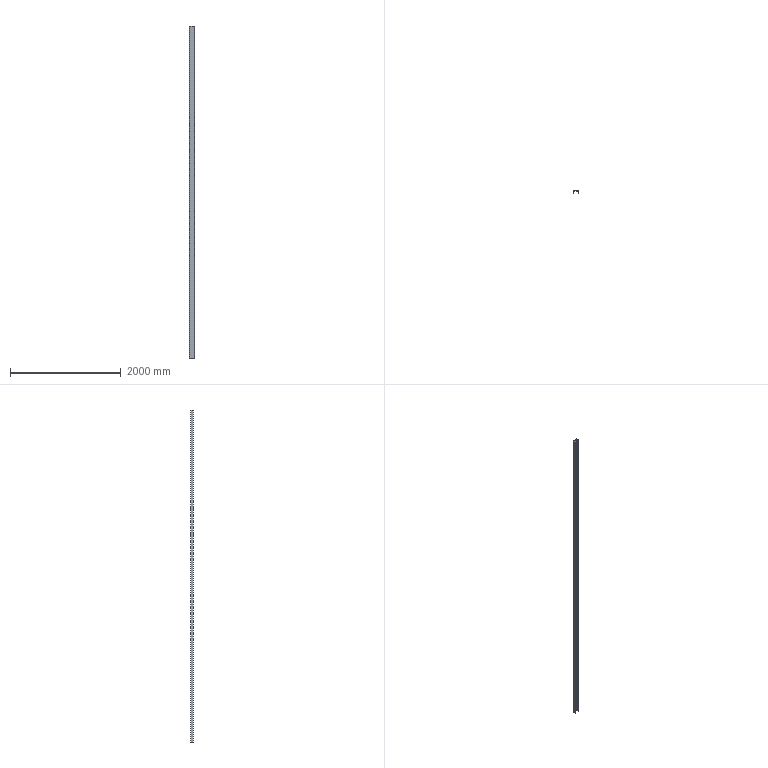Part | SolidWorks | features Extrusion 1 | 1 solid | 14 faces | box 100 x 50 x 6000 mm | volume 7666640 mm3 | plane 10 | cylinder 4 | commonest cylinder face diameters 4 x2 10 x2
STEP:
#1=CARTESIAN_POINT('',(0.,0.,0.));
#2=VERTEX_POINT('',#1);
#3=CARTESIAN_POINT('',(2.549,0.,0.));
#4=VERTEX_POINT('',#3);
#5=CARTESIAN_POINT('',(0.,0.,0.));
#6=DIRECTION('',(1.,0.,0.));
#7=VECTOR('',#6,1000.);
#8=LINE('',#5,#7);
#9=EDGE_CURVE('',#2,#4,#8,.T.);
#10=ORIENTED_EDGE('',*,*,#9,.T.);
#11=CARTESIAN_POINT('',(2.549,0.,6000.));
#12=VERTEX_POINT('',#11);
#13=CARTESIAN_POINT('',(2.549,0.,6000.));
#14=DIRECTION('',(0.,0.,-1.));
#15=VECTOR('',#14,1000.);
#16=LINE('',#13,#15);
#17=EDGE_CURVE('',#12,#4,#16,.T.);
#18=ORIENTED_EDGE('',*,*,#17,.F.);
#19=CARTESIAN_POINT('',(0.,0.,6000.));
#20=VERTEX_POINT('',#19);
#21=CARTESIAN_POINT('',(0.,0.,6000.));
#22=DIRECTION('',(1.,0.,0.));
#23=VECTOR('',#22,1000.);
#24=LINE('',#21,#23);
#25=EDGE_CURVE('',#20,#12,#24,.T.);
#26=ORIENTED_EDGE('',*,*,#25,.F.);
#27=CARTESIAN_POINT('',(0.,0.,6000.));
#28=DIRECTION('',(0.,0.,-1.));
#29=VECTOR('',#28,1000.);
#30=LINE('',#27,#29);
#31=EDGE_CURVE('',#20,#2,#30,.T.);
#32=ORIENTED_EDGE('',*,*,#31,.T.);
#33=EDGE_LOOP('',(#10,#18,#26,#32));
#34=FACE_OUTER_BOUND('',#33,.T.);
#35=CARTESIAN_POINT('',(0.,0.,6000.));
#36=DIRECTION('',(0.,1.,0.));
#37=DIRECTION('',(0.,0.,1.));
#38=AXIS2_PLACEMENT_3D('',#35,#36,#37);
#39=PLANE('',#38);
#40=ADVANCED_FACE('',(#34),#39,.F.);
#41=CARTESIAN_POINT('',(4.536,1.773,0.));
#42=VERTEX_POINT('',#41);
#43=CARTESIAN_POINT('',(2.549,2.,0.));
#44=DIRECTION('',(0.,0.,1.));
#45=DIRECTION('',(-1.,0.,0.));
#46=AXIS2_PLACEMENT_3D('',#43,#44,#45);
#47=CIRCLE('',#46,2.);
#48=EDGE_CURVE('',#4,#42,#47,.T.);
#49=ORIENTED_EDGE('',*,*,#48,.T.);
#50=CARTESIAN_POINT('',(4.536,1.773,6000.));
#51=VERTEX_POINT('',#50);
#52=CARTESIAN_POINT('',(4.536,1.773,6000.));
#53=DIRECTION('',(0.,0.,-1.));
#54=VECTOR('',#53,1000.);
#55=LINE('',#52,#54);
#56=EDGE_CURVE('',#51,#42,#55,.T.);
#57=ORIENTED_EDGE('',*,*,#56,.F.);
#58=CARTESIAN_POINT('',(2.549,2.,6000.));
#59=DIRECTION('',(0.,0.,1.));
#60=DIRECTION('',(-1.,0.,0.));
#61=AXIS2_PLACEMENT_3D('',#58,#59,#60);
#62=CIRCLE('',#61,2.);
#63=EDGE_CURVE('',#12,#51,#62,.T.);
#64=ORIENTED_EDGE('',*,*,#63,.F.);
#65=ORIENTED_EDGE('',*,*,#17,.T.);
#66=EDGE_LOOP('',(#49,#57,#64,#65));
#67=FACE_OUTER_BOUND('',#66,.T.);
#68=CARTESIAN_POINT('',(2.549,2.,6000.));
#69=DIRECTION('',(0.,0.,-1.));
#70=DIRECTION('',(-1.,0.,0.));
#71=AXIS2_PLACEMENT_3D('',#68,#69,#70);
#72=CYLINDRICAL_SURFACE('',#71,2.);
#73=ADVANCED_FACE('',(#67),#72,.T.);
#74=CARTESIAN_POINT('',(8.753,38.724,0.));
#75=VERTEX_POINT('',#74);
#76=CARTESIAN_POINT('',(4.536,1.773,0.));
#77=DIRECTION('',(0.1134,0.9936,0.));
#78=VECTOR('',#77,1000.);
#79=LINE('',#76,#78);
#80=EDGE_CURVE('',#42,#75,#79,.T.);
#81=ORIENTED_EDGE('',*,*,#80,.T.);
#82=CARTESIAN_POINT('',(8.753,38.724,6000.));
#83=VERTEX_POINT('',#82);
#84=CARTESIAN_POINT('',(8.753,38.724,6000.));
#85=DIRECTION('',(0.,0.,-1.));
#86=VECTOR('',#85,1000.);
#87=LINE('',#84,#86);
#88=EDGE_CURVE('',#83,#75,#87,.T.);
#89=ORIENTED_EDGE('',*,*,#88,.F.);
#90=CARTESIAN_POINT('',(4.536,1.773,6000.));
#91=DIRECTION('',(0.1134,0.9936,0.));
#92=VECTOR('',#91,1000.);
#93=LINE('',#90,#92);
#94=EDGE_CURVE('',#51,#83,#93,.T.);
#95=ORIENTED_EDGE('',*,*,#94,.F.);
#96=ORIENTED_EDGE('',*,*,#56,.T.);
#97=EDGE_LOOP('',(#81,#89,#95,#96));
#98=FACE_OUTER_BOUND('',#97,.T.);
#99=CARTESIAN_POINT('',(4.536,1.773,6000.));
#100=DIRECTION('',(-0.9936,0.1134,0.));
#101=DIRECTION('',(-0.1134,-0.9936,0.));
#102=AXIS2_PLACEMENT_3D('',#99,#100,#101);
#103=PLANE('',#102);
#104=ADVANCED_FACE('',(#98),#103,.F.);
#105=CARTESIAN_POINT('',(13.72,43.157,0.));
#106=VERTEX_POINT('',#105);
#107=CARTESIAN_POINT('',(13.72,38.157,0.));
#108=DIRECTION('',(0.,0.,-1.));
#109=DIRECTION('',(-1.,0.,0.));
#110=AXIS2_PLACEMENT_3D('',#107,#108,#109);
#111=CIRCLE('',#110,5.);
#112=EDGE_CURVE('',#75,#106,#111,.T.);
#113=ORIENTED_EDGE('',*,*,#112,.T.);
#114=CARTESIAN_POINT('',(13.72,43.157,6000.));
#115=VERTEX_POINT('',#114);
#116=CARTESIAN_POINT('',(13.72,43.157,6000.));
#117=DIRECTION('',(0.,0.,-1.));
#118=VECTOR('',#117,1000.);
#119=LINE('',#116,#118);
#120=EDGE_CURVE('',#115,#106,#119,.T.);
#121=ORIENTED_EDGE('',*,*,#120,.F.);
#122=CARTESIAN_POINT('',(13.72,38.157,6000.));
#123=DIRECTION('',(0.,0.,-1.));
#124=DIRECTION('',(-1.,0.,0.));
#125=AXIS2_PLACEMENT_3D('',#122,#123,#124);
#126=CIRCLE('',#125,5.);
#127=EDGE_CURVE('',#83,#115,#126,.T.);
#128=ORIENTED_EDGE('',*,*,#127,.F.);
#129=ORIENTED_EDGE('',*,*,#88,.T.);
#130=EDGE_LOOP('',(#113,#121,#128,#129));
#131=FACE_OUTER_BOUND('',#130,.T.);
#132=CARTESIAN_POINT('',(13.72,38.157,6000.));
#133=DIRECTION('',(0.,0.,-1.));
#134=DIRECTION('',(-1.,0.,0.));
#135=AXIS2_PLACEMENT_3D('',#132,#133,#134);
#136=CYLINDRICAL_SURFACE('',#135,5.);
#137=ADVANCED_FACE('',(#131),#136,.F.);
#138=CARTESIAN_POINT('',(86.28,43.157,0.));
#139=VERTEX_POINT('',#138);
#140=CARTESIAN_POINT('',(13.72,43.157,0.));
#141=DIRECTION('',(1.,0.,0.));
#142=VECTOR('',#141,1000.);
#143=LINE('',#140,#142);
#144=EDGE_CURVE('',#106,#139,#143,.T.);
#145=ORIENTED_EDGE('',*,*,#144,.T.);
#146=CARTESIAN_POINT('',(86.28,43.157,6000.));
#147=VERTEX_POINT('',#146);
#148=CARTESIAN_POINT('',(86.28,43.157,6000.));
#149=DIRECTION('',(0.,0.,-1.));
#150=VECTOR('',#149,1000.);
#151=LINE('',#148,#150);
#152=EDGE_CURVE('',#147,#139,#151,.T.);
#153=ORIENTED_EDGE('',*,*,#152,.F.);
#154=CARTESIAN_POINT('',(13.72,43.157,6000.));
#155=DIRECTION('',(1.,0.,0.));
#156=VECTOR('',#155,1000.);
#157=LINE('',#154,#156);
#158=EDGE_CURVE('',#115,#147,#157,.T.);
#159=ORIENTED_EDGE('',*,*,#158,.F.);
#160=ORIENTED_EDGE('',*,*,#120,.T.);
#161=EDGE_LOOP('',(#145,#153,#159,#160));
#162=FACE_OUTER_BOUND('',#161,.T.);
#163=CARTESIAN_POINT('',(13.72,43.157,6000.));
#164=DIRECTION('',(0.,1.,0.));
#165=DIRECTION('',(-1.,0.,0.));
#166=AXIS2_PLACEMENT_3D('',#163,#164,#165);
#167=PLANE('',#166);
#168=ADVANCED_FACE('',(#162),#167,.F.);
#169=CARTESIAN_POINT('',(91.247,38.724,0.));
#170=VERTEX_POINT('',#169);
#171=CARTESIAN_POINT('',(86.28,38.157,0.));
#172=DIRECTION('',(0.,0.,-1.));
#173=DIRECTION('',(1.,0.,0.));
#174=AXIS2_PLACEMENT_3D('',#171,#172,#173);
#175=CIRCLE('',#174,5.);
#176=EDGE_CURVE('',#139,#170,#175,.T.);
#177=ORIENTED_EDGE('',*,*,#176,.T.);
#178=CARTESIAN_POINT('',(91.247,38.724,6000.));
#179=VERTEX_POINT('',#178);
#180=CARTESIAN_POINT('',(91.247,38.724,6000.));
#181=DIRECTION('',(0.,0.,-1.));
#182=VECTOR('',#181,1000.);
#183=LINE('',#180,#182);
#184=EDGE_CURVE('',#179,#170,#183,.T.);
#185=ORIENTED_EDGE('',*,*,#184,.F.);
#186=CARTESIAN_POINT('',(86.28,38.157,6000.));
#187=DIRECTION('',(0.,0.,-1.));
#188=DIRECTION('',(1.,0.,0.));
#189=AXIS2_PLACEMENT_3D('',#186,#187,#188);
#190=CIRCLE('',#189,5.);
#191=EDGE_CURVE('',#147,#179,#190,.T.);
#192=ORIENTED_EDGE('',*,*,#191,.F.);
#193=ORIENTED_EDGE('',*,*,#152,.T.);
#194=EDGE_LOOP('',(#177,#185,#192,#193));
#195=FACE_OUTER_BOUND('',#194,.T.);
#196=CARTESIAN_POINT('',(86.28,38.157,6000.));
#197=DIRECTION('',(0.,0.,-1.));
#198=DIRECTION('',(-1.,0.,0.));
#199=AXIS2_PLACEMENT_3D('',#196,#197,#198);
#200=CYLINDRICAL_SURFACE('',#199,5.);
#201=ADVANCED_FACE('',(#195),#200,.F.);
#202=CARTESIAN_POINT('',(95.464,1.773,0.));
#203=VERTEX_POINT('',#202);
#204=CARTESIAN_POINT('',(95.464,1.773,0.));
#205=DIRECTION('',(0.1134,-0.9936,0.));
#206=VECTOR('',#205,1000.);
#207=LINE('',#204,#206);
#208=EDGE_CURVE('',#170,#203,#207,.T.);
#209=ORIENTED_EDGE('',*,*,#208,.T.);
#210=CARTESIAN_POINT('',(95.464,1.773,6000.));
#211=VERTEX_POINT('',#210);
#212=CARTESIAN_POINT('',(95.464,1.773,6000.));
#213=DIRECTION('',(0.,0.,-1.));
#214=VECTOR('',#213,1000.);
#215=LINE('',#212,#214);
#216=EDGE_CURVE('',#211,#203,#215,.T.);
#217=ORIENTED_EDGE('',*,*,#216,.F.);
#218=CARTESIAN_POINT('',(95.464,1.773,6000.));
#219=DIRECTION('',(0.1134,-0.9936,0.));
#220=VECTOR('',#219,1000.);
#221=LINE('',#218,#220);
#222=EDGE_CURVE('',#179,#211,#221,.T.);
#223=ORIENTED_EDGE('',*,*,#222,.F.);
#224=ORIENTED_EDGE('',*,*,#184,.T.);
#225=EDGE_LOOP('',(#209,#217,#223,#224));
#226=FACE_OUTER_BOUND('',#225,.T.);
#227=CARTESIAN_POINT('',(95.464,1.773,6000.));
#228=DIRECTION('',(0.9936,0.1134,0.));
#229=DIRECTION('',(-0.1134,0.9936,0.));
#230=AXIS2_PLACEMENT_3D('',#227,#228,#229);
#231=PLANE('',#230);
#232=ADVANCED_FACE('',(#226),#231,.F.);
#233=CARTESIAN_POINT('',(97.451,0.,0.));
#234=VERTEX_POINT('',#233);
#235=CARTESIAN_POINT('',(97.451,2.,0.));
#236=DIRECTION('',(0.,0.,1.));
#237=DIRECTION('',(1.,0.,0.));
#238=AXIS2_PLACEMENT_3D('',#235,#236,#237);
#239=CIRCLE('',#238,2.);
#240=EDGE_CURVE('',#203,#234,#239,.T.);
#241=ORIENTED_EDGE('',*,*,#240,.T.);
#242=CARTESIAN_POINT('',(97.451,0.,6000.));
#243=VERTEX_POINT('',#242);
#244=CARTESIAN_POINT('',(97.451,0.,6000.));
#245=DIRECTION('',(0.,0.,-1.));
#246=VECTOR('',#245,1000.);
#247=LINE('',#244,#246);
#248=EDGE_CURVE('',#243,#234,#247,.T.);
#249=ORIENTED_EDGE('',*,*,#248,.F.);
#250=CARTESIAN_POINT('',(97.451,2.,6000.));
#251=DIRECTION('',(0.,0.,1.));
#252=DIRECTION('',(1.,0.,0.));
#253=AXIS2_PLACEMENT_3D('',#250,#251,#252);
#254=CIRCLE('',#253,2.);
#255=EDGE_CURVE('',#211,#243,#254,.T.);
#256=ORIENTED_EDGE('',*,*,#255,.F.);
#257=ORIENTED_EDGE('',*,*,#216,.T.);
#258=EDGE_LOOP('',(#241,#249,#256,#257));
#259=FACE_OUTER_BOUND('',#258,.T.);
#260=CARTESIAN_POINT('',(97.451,2.,6000.));
#261=DIRECTION('',(0.,0.,-1.));
#262=DIRECTION('',(-1.,0.,0.));
#263=AXIS2_PLACEMENT_3D('',#260,#261,#262);
#264=CYLINDRICAL_SURFACE('',#263,2.);
#265=ADVANCED_FACE('',(#259),#264,.T.);
#266=CARTESIAN_POINT('',(100.,0.,0.));
#267=VERTEX_POINT('',#266);
#268=CARTESIAN_POINT('',(100.,0.,0.));
#269=DIRECTION('',(1.,0.,0.));
#270=VECTOR('',#269,1000.);
#271=LINE('',#268,#270);
#272=EDGE_CURVE('',#234,#267,#271,.T.);
#273=ORIENTED_EDGE('',*,*,#272,.T.);
#274=CARTESIAN_POINT('',(100.,0.,6000.));
#275=VERTEX_POINT('',#274);
#276=CARTESIAN_POINT('',(100.,0.,6000.));
#277=DIRECTION('',(0.,0.,-1.));
#278=VECTOR('',#277,1000.);
#279=LINE('',#276,#278);
#280=EDGE_CURVE('',#275,#267,#279,.T.);
#281=ORIENTED_EDGE('',*,*,#280,.F.);
#282=CARTESIAN_POINT('',(100.,0.,6000.));
#283=DIRECTION('',(1.,0.,0.));
#284=VECTOR('',#283,1000.);
#285=LINE('',#282,#284);
#286=EDGE_CURVE('',#243,#275,#285,.T.);
#287=ORIENTED_EDGE('',*,*,#286,.F.);
#288=ORIENTED_EDGE('',*,*,#248,.T.);
#289=EDGE_LOOP('',(#273,#281,#287,#288));
#290=FACE_OUTER_BOUND('',#289,.T.);
#291=CARTESIAN_POINT('',(100.,0.,6000.));
#292=DIRECTION('',(0.,1.,0.));
#293=DIRECTION('',(-1.,0.,0.));
#294=AXIS2_PLACEMENT_3D('',#291,#292,#293);
#295=PLANE('',#294);
#296=ADVANCED_FACE('',(#290),#295,.F.);
#297=CARTESIAN_POINT('',(100.,50.,0.));
#298=VERTEX_POINT('',#297);
#299=CARTESIAN_POINT('',(100.,50.,0.));
#300=DIRECTION('',(0.,1.,0.));
#301=VECTOR('',#300,1000.);
#302=LINE('',#299,#301);
#303=EDGE_CURVE('',#267,#298,#302,.T.);
#304=ORIENTED_EDGE('',*,*,#303,.T.);
#305=CARTESIAN_POINT('',(100.,50.,6000.));
#306=VERTEX_POINT('',#305);
#307=CARTESIAN_POINT('',(100.,50.,6000.));
#308=DIRECTION('',(0.,0.,-1.));
#309=VECTOR('',#308,1000.);
#310=LINE('',#307,#309);
#311=EDGE_CURVE('',#306,#298,#310,.T.);
#312=ORIENTED_EDGE('',*,*,#311,.F.);
#313=CARTESIAN_POINT('',(100.,50.,6000.));
#314=DIRECTION('',(0.,1.,0.));
#315=VECTOR('',#314,1000.);
#316=LINE('',#313,#315);
#317=EDGE_CURVE('',#275,#306,#316,.T.);
#318=ORIENTED_EDGE('',*,*,#317,.F.);
#319=ORIENTED_EDGE('',*,*,#280,.T.);
#320=EDGE_LOOP('',(#304,#312,#318,#319));
#321=FACE_OUTER_BOUND('',#320,.T.);
#322=CARTESIAN_POINT('',(100.,50.,6000.));
#323=DIRECTION('',(-1.,0.,0.));
#324=DIRECTION('',(0.,-1.,0.));
#325=AXIS2_PLACEMENT_3D('',#322,#323,#324);
#326=PLANE('',#325);
#327=ADVANCED_FACE('',(#321),#326,.F.);
#328=CARTESIAN_POINT('',(0.,50.,0.));
#329=VERTEX_POINT('',#328);
#330=CARTESIAN_POINT('',(0.,50.,0.));
#331=DIRECTION('',(-1.,0.,0.));
#332=VECTOR('',#331,1000.);
#333=LINE('',#330,#332);
#334=EDGE_CURVE('',#298,#329,#333,.T.);
#335=ORIENTED_EDGE('',*,*,#334,.T.);
#336=CARTESIAN_POINT('',(0.,50.,6000.));
#337=VERTEX_POINT('',#336);
#338=CARTESIAN_POINT('',(0.,50.,6000.));
#339=DIRECTION('',(0.,0.,-1.));
#340=VECTOR('',#339,1000.);
#341=LINE('',#338,#340);
#342=EDGE_CURVE('',#337,#329,#341,.T.);
#343=ORIENTED_EDGE('',*,*,#342,.F.);
#344=CARTESIAN_POINT('',(0.,50.,6000.));
#345=DIRECTION('',(-1.,0.,0.));
#346=VECTOR('',#345,1000.);
#347=LINE('',#344,#346);
#348=EDGE_CURVE('',#306,#337,#347,.T.);
#349=ORIENTED_EDGE('',*,*,#348,.F.);
#350=ORIENTED_EDGE('',*,*,#311,.T.);
#351=EDGE_LOOP('',(#335,#343,#349,#350));
#352=FACE_OUTER_BOUND('',#351,.T.);
#353=CARTESIAN_POINT('',(0.,50.,6000.));
#354=DIRECTION('',(0.,-1.,0.));
#355=DIRECTION('',(1.,0.,0.));
#356=AXIS2_PLACEMENT_3D('',#353,#354,#355);
#357=PLANE('',#356);
#358=ADVANCED_FACE('',(#352),#357,.F.);
#359=CARTESIAN_POINT('',(0.,0.,0.));
#360=DIRECTION('',(0.,-1.,0.));
#361=VECTOR('',#360,1000.);
#362=LINE('',#359,#361);
#363=EDGE_CURVE('',#329,#2,#362,.T.);
#364=ORIENTED_EDGE('',*,*,#363,.T.);
#365=ORIENTED_EDGE('',*,*,#31,.F.);
#366=CARTESIAN_POINT('',(0.,0.,6000.));
#367=DIRECTION('',(0.,-1.,0.));
#368=VECTOR('',#367,1000.);
#369=LINE('',#366,#368);
#370=EDGE_CURVE('',#337,#20,#369,.T.);
#371=ORIENTED_EDGE('',*,*,#370,.F.);
#372=ORIENTED_EDGE('',*,*,#342,.T.);
#373=EDGE_LOOP('',(#364,#365,#371,#372));
#374=FACE_OUTER_BOUND('',#373,.T.);
#375=CARTESIAN_POINT('',(0.,0.,6000.));
#376=DIRECTION('',(1.,0.,0.));
#377=DIRECTION('',(0.,0.,-1.));
#378=AXIS2_PLACEMENT_3D('',#375,#376,#377);
#379=PLANE('',#378);
#380=ADVANCED_FACE('',(#374),#379,.F.);
#381=ORIENTED_EDGE('',*,*,#25,.T.);
#382=ORIENTED_EDGE('',*,*,#63,.T.);
#383=ORIENTED_EDGE('',*,*,#94,.T.);
#384=ORIENTED_EDGE('',*,*,#127,.T.);
#385=ORIENTED_EDGE('',*,*,#158,.T.);
#386=ORIENTED_EDGE('',*,*,#191,.T.);
#387=ORIENTED_EDGE('',*,*,#222,.T.);
#388=ORIENTED_EDGE('',*,*,#255,.T.);
#389=ORIENTED_EDGE('',*,*,#286,.T.);
#390=ORIENTED_EDGE('',*,*,#317,.T.);
#391=ORIENTED_EDGE('',*,*,#348,.T.);
#392=ORIENTED_EDGE('',*,*,#370,.T.);
#393=EDGE_LOOP('',(#381,#382,#383,#384,#385,#386,#387,#388,#389,#390,#391,#392));
#394=FACE_OUTER_BOUND('',#393,.T.);
#395=CARTESIAN_POINT('',(2.549,2.,6000.));
#396=DIRECTION('',(0.,0.,-1.));
#397=DIRECTION('',(-1.,0.,0.));
#398=AXIS2_PLACEMENT_3D('',#395,#396,#397);
#399=PLANE('',#398);
#400=ADVANCED_FACE('',(#394),#399,.F.);
#401=ORIENTED_EDGE('',*,*,#9,.F.);
#402=ORIENTED_EDGE('',*,*,#363,.F.);
#403=ORIENTED_EDGE('',*,*,#334,.F.);
#404=ORIENTED_EDGE('',*,*,#303,.F.);
#405=ORIENTED_EDGE('',*,*,#272,.F.);
#406=ORIENTED_EDGE('',*,*,#240,.F.);
#407=ORIENTED_EDGE('',*,*,#208,.F.);
#408=ORIENTED_EDGE('',*,*,#176,.F.);
#409=ORIENTED_EDGE('',*,*,#144,.F.);
#410=ORIENTED_EDGE('',*,*,#112,.F.);
#411=ORIENTED_EDGE('',*,*,#80,.F.);
#412=ORIENTED_EDGE('',*,*,#48,.F.);
#413=EDGE_LOOP('',(#401,#402,#403,#404,#405,#406,#407,#408,#409,#410,#411,#412));
#414=FACE_OUTER_BOUND('',#413,.T.);
#415=CARTESIAN_POINT('',(2.549,2.,0.));
#416=DIRECTION('',(0.,0.,-1.));
#417=DIRECTION('',(-1.,0.,0.));
#418=AXIS2_PLACEMENT_3D('',#415,#416,#417);
#419=PLANE('',#418);
#420=ADVANCED_FACE('',(#414),#419,.T.);
#421=CLOSED_SHELL('',(#40,#73,#104,#137,#168,#201,#232,#265,#296,#327,#358,#380,#400,#420));
#422=MANIFOLD_SOLID_BREP('',#421);
#423=CARTESIAN_POINT('',(0.,0.,0.));
#424=DIRECTION('',(0.,0.,1.));
#425=DIRECTION('',(1.,0.,0.));
#426=AXIS2_PLACEMENT_3D('',#423,#424,#425);
#427=(LENGTH_UNIT()NAMED_UNIT(*)SI_UNIT(.MILLI.,.METRE.));
#428=UNCERTAINTY_MEASURE_WITH_UNIT(LENGTH_MEASURE(0.00001),#427,'','');
#429=(NAMED_UNIT(*)PLANE_ANGLE_UNIT()SI_UNIT($,.RADIAN.));
#430=(NAMED_UNIT(*)SI_UNIT($,.STERADIAN.)SOLID_ANGLE_UNIT());
#431=(GEOMETRIC_REPRESENTATION_CONTEXT(3)GLOBAL_UNCERTAINTY_ASSIGNED_CONTEXT((#428))GLOBAL_UNIT_ASSIGNED_CONTEXT((#427,#429,#430))REPRESENTATION_CONTEXT('',''));
#432=ADVANCED_BREP_SHAPE_REPRESENTATION('',(#422,#426),#431);